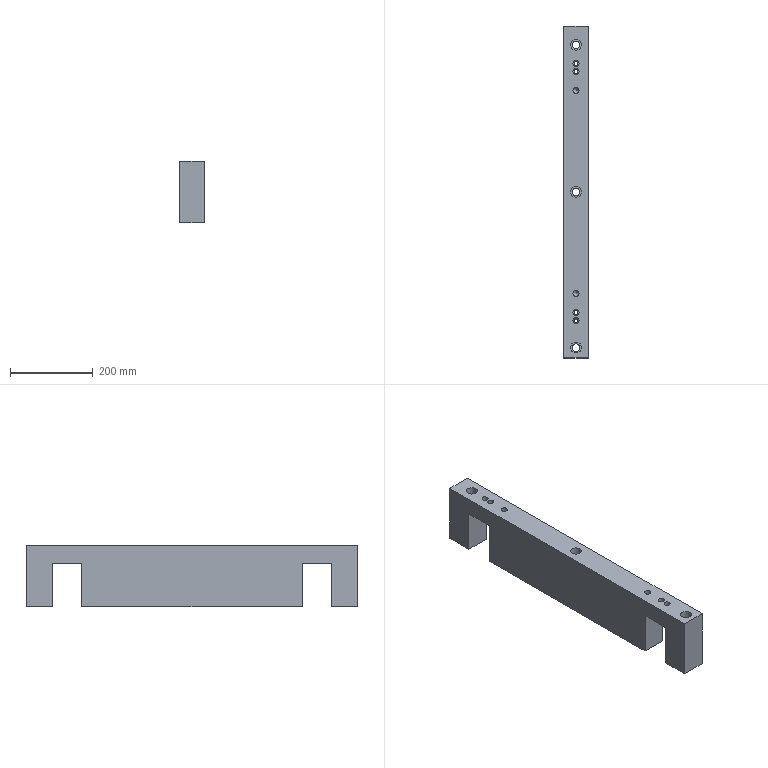Part | STEP file | lll_id2314_x_t | 1 solid | 39 faces | box 60 x 800 x 147.5 mm | volume 5972618 mm3 | plane 21 | cylinder 16 | cone 2 | commonest cylinder face diameters 9.009 x4 14.508 x4 18.009 x3 26.008 x3 14.506 x2
STEP:
#1=CARTESIAN_POINT('',(2157.253,-244.498,370.));
#2=VERTEX_POINT('',#1);
#3=CARTESIAN_POINT('',(2150.,-244.498,370.));
#4=DIRECTION('',(0.,0.,-1.));
#5=DIRECTION('',(1.,0.,0.));
#6=AXIS2_PLACEMENT_3D('',#3,#4,#5);
#7=CIRCLE('',#6,7.253);
#8=EDGE_CURVE('',#2,#2,#7,.T.);
#9=ORIENTED_EDGE('',*,*,#8,.T.);
#10=EDGE_LOOP('',(#9));
#11=FACE_BOUND('',#10,.T.);
#12=CARTESIAN_POINT('',(2157.253,244.498,370.));
#13=VERTEX_POINT('',#12);
#14=CARTESIAN_POINT('',(2150.,244.498,370.));
#15=DIRECTION('',(0.,0.,1.));
#16=DIRECTION('',(1.,0.,0.));
#17=AXIS2_PLACEMENT_3D('',#14,#15,#16);
#18=CIRCLE('',#17,7.253);
#19=EDGE_CURVE('',#13,#13,#18,.T.);
#20=ORIENTED_EDGE('',*,*,#19,.F.);
#21=EDGE_LOOP('',(#20));
#22=FACE_BOUND('',#21,.T.);
#23=CARTESIAN_POINT('',(2163.004,355.,370.));
#24=VERTEX_POINT('',#23);
#25=CARTESIAN_POINT('',(2150.,355.,370.));
#26=DIRECTION('',(0.,0.,-1.));
#27=DIRECTION('',(1.,0.,0.));
#28=AXIS2_PLACEMENT_3D('',#25,#26,#27);
#29=CIRCLE('',#28,13.004);
#30=EDGE_CURVE('',#24,#24,#29,.T.);
#31=ORIENTED_EDGE('',*,*,#30,.T.);
#32=EDGE_LOOP('',(#31));
#33=FACE_BOUND('',#32,.T.);
#34=CARTESIAN_POINT('',(2180.,400.,370.));
#35=VERTEX_POINT('',#34);
#36=CARTESIAN_POINT('',(2120.,400.,370.));
#37=VERTEX_POINT('',#36);
#38=CARTESIAN_POINT('',(6090.,400.,370.));
#39=DIRECTION('',(-1.,0.,0.));
#40=VECTOR('',#39,1.);
#41=LINE('',#38,#40);
#42=EDGE_CURVE('',#35,#37,#41,.T.);
#43=ORIENTED_EDGE('',*,*,#42,.T.);
#44=CARTESIAN_POINT('',(2120.,-400.,370.));
#45=VERTEX_POINT('',#44);
#46=CARTESIAN_POINT('',(2120.,600.,370.));
#47=DIRECTION('',(0.,-1.,0.));
#48=VECTOR('',#47,1.);
#49=LINE('',#46,#48);
#50=EDGE_CURVE('',#37,#45,#49,.T.);
#51=ORIENTED_EDGE('',*,*,#50,.T.);
#52=CARTESIAN_POINT('',(2180.,-400.,370.));
#53=VERTEX_POINT('',#52);
#54=CARTESIAN_POINT('',(2120.,-400.,370.));
#55=DIRECTION('',(1.,0.,0.));
#56=VECTOR('',#55,1.);
#57=LINE('',#54,#56);
#58=EDGE_CURVE('',#45,#53,#57,.T.);
#59=ORIENTED_EDGE('',*,*,#58,.T.);
#60=CARTESIAN_POINT('',(2180.,1.,370.));
#61=DIRECTION('',(0.,1.,0.));
#62=VECTOR('',#61,1.);
#63=LINE('',#60,#62);
#64=EDGE_CURVE('',#53,#35,#63,.T.);
#65=ORIENTED_EDGE('',*,*,#64,.T.);
#66=EDGE_LOOP('',(#43,#51,#59,#65));
#67=FACE_BOUND('',#66,.T.);
#68=CARTESIAN_POINT('',(2157.254,310.,370.));
#69=VERTEX_POINT('',#68);
#70=CARTESIAN_POINT('',(2150.,310.,370.));
#71=DIRECTION('',(0.,0.,-1.));
#72=DIRECTION('',(1.,0.,0.));
#73=AXIS2_PLACEMENT_3D('',#70,#71,#72);
#74=CIRCLE('',#73,7.254);
#75=EDGE_CURVE('',#69,#69,#74,.T.);
#76=ORIENTED_EDGE('',*,*,#75,.T.);
#77=EDGE_LOOP('',(#76));
#78=FACE_BOUND('',#77,.T.);
#79=CARTESIAN_POINT('',(2157.254,290.,370.));
#80=VERTEX_POINT('',#79);
#81=CARTESIAN_POINT('',(2150.,290.,370.));
#82=DIRECTION('',(0.,0.,-1.));
#83=DIRECTION('',(1.,0.,0.));
#84=AXIS2_PLACEMENT_3D('',#81,#82,#83);
#85=CIRCLE('',#84,7.254);
#86=EDGE_CURVE('',#80,#80,#85,.T.);
#87=ORIENTED_EDGE('',*,*,#86,.T.);
#88=EDGE_LOOP('',(#87));
#89=FACE_BOUND('',#88,.T.);
#90=CARTESIAN_POINT('',(2157.254,-290.498,370.));
#91=VERTEX_POINT('',#90);
#92=CARTESIAN_POINT('',(2150.,-290.498,370.));
#93=DIRECTION('',(0.,0.,-1.));
#94=DIRECTION('',(1.,0.,0.));
#95=AXIS2_PLACEMENT_3D('',#92,#93,#94);
#96=CIRCLE('',#95,7.254);
#97=EDGE_CURVE('',#91,#91,#96,.T.);
#98=ORIENTED_EDGE('',*,*,#97,.T.);
#99=EDGE_LOOP('',(#98));
#100=FACE_BOUND('',#99,.T.);
#101=CARTESIAN_POINT('',(2157.254,-310.498,370.));
#102=VERTEX_POINT('',#101);
#103=CARTESIAN_POINT('',(2150.,-310.498,370.));
#104=DIRECTION('',(0.,0.,-1.));
#105=DIRECTION('',(1.,0.,0.));
#106=AXIS2_PLACEMENT_3D('',#103,#104,#105);
#107=CIRCLE('',#106,7.254);
#108=EDGE_CURVE('',#102,#102,#107,.T.);
#109=ORIENTED_EDGE('',*,*,#108,.T.);
#110=EDGE_LOOP('',(#109));
#111=FACE_BOUND('',#110,.T.);
#112=CARTESIAN_POINT('',(2163.004,0.,370.));
#113=VERTEX_POINT('',#112);
#114=CARTESIAN_POINT('',(2150.,0.,370.));
#115=DIRECTION('',(0.,0.,-1.));
#116=DIRECTION('',(1.,0.,0.));
#117=AXIS2_PLACEMENT_3D('',#114,#115,#116);
#118=CIRCLE('',#117,13.004);
#119=EDGE_CURVE('',#113,#113,#118,.T.);
#120=ORIENTED_EDGE('',*,*,#119,.T.);
#121=EDGE_LOOP('',(#120));
#122=FACE_BOUND('',#121,.T.);
#123=CARTESIAN_POINT('',(2163.004,-375.,370.));
#124=VERTEX_POINT('',#123);
#125=CARTESIAN_POINT('',(2150.,-375.,370.));
#126=DIRECTION('',(0.,0.,1.));
#127=DIRECTION('',(1.,0.,0.));
#128=AXIS2_PLACEMENT_3D('',#125,#126,#127);
#129=CIRCLE('',#128,13.004);
#130=EDGE_CURVE('',#124,#124,#129,.T.);
#131=ORIENTED_EDGE('',*,*,#130,.F.);
#132=EDGE_LOOP('',(#131));
#133=FACE_BOUND('',#132,.T.);
#134=CARTESIAN_POINT('',(-66.315,1.,370.));
#135=DIRECTION('',(0.,0.,-1.));
#136=DIRECTION('',(1.,0.,0.));
#137=AXIS2_PLACEMENT_3D('',#134,#135,#136);
#138=PLANE('',#137);
#139=ADVANCED_FACE('',(#11,#22,#33,#67,#78,#89,#100,#111,#122,#133),#138,.F.);
#140=CARTESIAN_POINT('',(2140.995,0.,222.5));
#141=VERTEX_POINT('',#140);
#142=CARTESIAN_POINT('',(2150.,0.,222.5));
#143=DIRECTION('',(0.,0.,-1.));
#144=DIRECTION('',(-1.,0.,0.));
#145=AXIS2_PLACEMENT_3D('',#142,#143,#144);
#146=CIRCLE('',#145,9.005);
#147=EDGE_CURVE('',#141,#141,#146,.T.);
#148=ORIENTED_EDGE('',*,*,#147,.F.);
#149=EDGE_LOOP('',(#148));
#150=FACE_BOUND('',#149,.T.);
#151=CARTESIAN_POINT('',(2180.,265.249,222.5));
#152=VERTEX_POINT('',#151);
#153=CARTESIAN_POINT('',(2120.,265.249,222.5));
#154=VERTEX_POINT('',#153);
#155=CARTESIAN_POINT('',(-66.315,265.249,222.5));
#156=DIRECTION('',(-1.,0.,0.));
#157=VECTOR('',#156,1.);
#158=LINE('',#155,#157);
#159=EDGE_CURVE('',#152,#154,#158,.T.);
#160=ORIENTED_EDGE('',*,*,#159,.F.);
#161=CARTESIAN_POINT('',(2180.,-265.249,222.5));
#162=VERTEX_POINT('',#161);
#163=CARTESIAN_POINT('',(2180.,1.,222.5));
#164=DIRECTION('',(0.,-1.,0.));
#165=VECTOR('',#164,1.);
#166=LINE('',#163,#165);
#167=EDGE_CURVE('',#152,#162,#166,.T.);
#168=ORIENTED_EDGE('',*,*,#167,.T.);
#169=CARTESIAN_POINT('',(2120.,-265.249,222.5));
#170=VERTEX_POINT('',#169);
#171=CARTESIAN_POINT('',(-66.315,-265.249,222.5));
#172=DIRECTION('',(1.,0.,0.));
#173=VECTOR('',#172,1.);
#174=LINE('',#171,#173);
#175=EDGE_CURVE('',#170,#162,#174,.T.);
#176=ORIENTED_EDGE('',*,*,#175,.F.);
#177=CARTESIAN_POINT('',(2120.,600.,222.5));
#178=DIRECTION('',(0.,-1.,0.));
#179=VECTOR('',#178,1.);
#180=LINE('',#177,#179);
#181=EDGE_CURVE('',#154,#170,#180,.T.);
#182=ORIENTED_EDGE('',*,*,#181,.F.);
#183=EDGE_LOOP('',(#160,#168,#176,#182));
#184=FACE_BOUND('',#183,.T.);
#185=CARTESIAN_POINT('',(-66.315,1.,222.5));
#186=DIRECTION('',(0.,0.,-1.));
#187=DIRECTION('',(1.,0.,0.));
#188=AXIS2_PLACEMENT_3D('',#185,#186,#187);
#189=PLANE('',#188);
#190=ADVANCED_FACE('',(#150,#184),#189,.T.);
#191=CARTESIAN_POINT('',(2140.995,355.,222.5));
#192=VERTEX_POINT('',#191);
#193=CARTESIAN_POINT('',(2150.,355.,222.5));
#194=DIRECTION('',(0.,0.,-1.));
#195=DIRECTION('',(-1.,0.,0.));
#196=AXIS2_PLACEMENT_3D('',#193,#194,#195);
#197=CIRCLE('',#196,9.005);
#198=EDGE_CURVE('',#192,#192,#197,.T.);
#199=ORIENTED_EDGE('',*,*,#198,.F.);
#200=EDGE_LOOP('',(#199));
#201=FACE_BOUND('',#200,.T.);
#202=CARTESIAN_POINT('',(2120.,335.249,222.5));
#203=VERTEX_POINT('',#202);
#204=CARTESIAN_POINT('',(2180.,335.249,222.5));
#205=VERTEX_POINT('',#204);
#206=CARTESIAN_POINT('',(-66.315,335.249,222.5));
#207=DIRECTION('',(1.,0.,0.));
#208=VECTOR('',#207,1.);
#209=LINE('',#206,#208);
#210=EDGE_CURVE('',#203,#205,#209,.T.);
#211=ORIENTED_EDGE('',*,*,#210,.F.);
#212=CARTESIAN_POINT('',(2120.,400.,222.5));
#213=VERTEX_POINT('',#212);
#214=CARTESIAN_POINT('',(2120.,600.,222.5));
#215=DIRECTION('',(0.,-1.,0.));
#216=VECTOR('',#215,1.);
#217=LINE('',#214,#216);
#218=EDGE_CURVE('',#213,#203,#217,.T.);
#219=ORIENTED_EDGE('',*,*,#218,.F.);
#220=CARTESIAN_POINT('',(2180.,400.,222.5));
#221=VERTEX_POINT('',#220);
#222=CARTESIAN_POINT('',(6090.,400.,222.5));
#223=DIRECTION('',(-1.,0.,0.));
#224=VECTOR('',#223,1.);
#225=LINE('',#222,#224);
#226=EDGE_CURVE('',#221,#213,#225,.T.);
#227=ORIENTED_EDGE('',*,*,#226,.F.);
#228=CARTESIAN_POINT('',(2180.,1.,222.5));
#229=DIRECTION('',(0.,-1.,0.));
#230=VECTOR('',#229,1.);
#231=LINE('',#228,#230);
#232=EDGE_CURVE('',#221,#205,#231,.T.);
#233=ORIENTED_EDGE('',*,*,#232,.T.);
#234=EDGE_LOOP('',(#211,#219,#227,#233));
#235=FACE_BOUND('',#234,.T.);
#236=CARTESIAN_POINT('',(-66.315,1.,222.5));
#237=DIRECTION('',(0.,0.,-1.));
#238=DIRECTION('',(1.,0.,0.));
#239=AXIS2_PLACEMENT_3D('',#236,#237,#238);
#240=PLANE('',#239);
#241=ADVANCED_FACE('',(#201,#235),#240,.T.);
#242=CARTESIAN_POINT('',(2140.995,-375.,222.5));
#243=VERTEX_POINT('',#242);
#244=CARTESIAN_POINT('',(2150.,-375.,222.5));
#245=DIRECTION('',(0.,0.,-1.));
#246=DIRECTION('',(-1.,0.,0.));
#247=AXIS2_PLACEMENT_3D('',#244,#245,#246);
#248=CIRCLE('',#247,9.005);
#249=EDGE_CURVE('',#243,#243,#248,.T.);
#250=ORIENTED_EDGE('',*,*,#249,.F.);
#251=EDGE_LOOP('',(#250));
#252=FACE_BOUND('',#251,.T.);
#253=CARTESIAN_POINT('',(2180.,-335.249,222.5));
#254=VERTEX_POINT('',#253);
#255=CARTESIAN_POINT('',(2120.,-335.249,222.5));
#256=VERTEX_POINT('',#255);
#257=CARTESIAN_POINT('',(-66.315,-335.249,222.5));
#258=DIRECTION('',(-1.,0.,0.));
#259=VECTOR('',#258,1.);
#260=LINE('',#257,#259);
#261=EDGE_CURVE('',#254,#256,#260,.T.);
#262=ORIENTED_EDGE('',*,*,#261,.F.);
#263=CARTESIAN_POINT('',(2180.,-400.,222.5));
#264=VERTEX_POINT('',#263);
#265=CARTESIAN_POINT('',(2180.,1.,222.5));
#266=DIRECTION('',(0.,-1.,0.));
#267=VECTOR('',#266,1.);
#268=LINE('',#265,#267);
#269=EDGE_CURVE('',#254,#264,#268,.T.);
#270=ORIENTED_EDGE('',*,*,#269,.T.);
#271=CARTESIAN_POINT('',(2120.,-400.,222.5));
#272=VERTEX_POINT('',#271);
#273=CARTESIAN_POINT('',(2120.,-400.,222.5));
#274=DIRECTION('',(1.,0.,0.));
#275=VECTOR('',#274,1.);
#276=LINE('',#273,#275);
#277=EDGE_CURVE('',#272,#264,#276,.T.);
#278=ORIENTED_EDGE('',*,*,#277,.F.);
#279=CARTESIAN_POINT('',(2120.,600.,222.5));
#280=DIRECTION('',(0.,-1.,0.));
#281=VECTOR('',#280,1.);
#282=LINE('',#279,#281);
#283=EDGE_CURVE('',#256,#272,#282,.T.);
#284=ORIENTED_EDGE('',*,*,#283,.F.);
#285=EDGE_LOOP('',(#262,#270,#278,#284));
#286=FACE_BOUND('',#285,.T.);
#287=CARTESIAN_POINT('',(-66.315,1.,222.5));
#288=DIRECTION('',(0.,0.,-1.));
#289=DIRECTION('',(1.,0.,0.));
#290=AXIS2_PLACEMENT_3D('',#287,#288,#289);
#291=PLANE('',#290);
#292=ADVANCED_FACE('',(#252,#286),#291,.T.);
#293=CARTESIAN_POINT('',(2120.,-335.249,326.5));
#294=VERTEX_POINT('',#293);
#295=CARTESIAN_POINT('',(2120.,-265.249,326.5));
#296=VERTEX_POINT('',#295);
#297=CARTESIAN_POINT('',(2120.,-50.498,326.5));
#298=DIRECTION('',(0.,1.,0.));
#299=VECTOR('',#298,1.);
#300=LINE('',#297,#299);
#301=EDGE_CURVE('',#294,#296,#300,.T.);
#302=ORIENTED_EDGE('',*,*,#301,.F.);
#303=CARTESIAN_POINT('',(2120.,-335.249,363.5));
#304=DIRECTION('',(0.,0.,1.));
#305=VECTOR('',#304,1.);
#306=LINE('',#303,#305);
#307=EDGE_CURVE('',#256,#294,#306,.T.);
#308=ORIENTED_EDGE('',*,*,#307,.F.);
#309=ORIENTED_EDGE('',*,*,#283,.T.);
#310=CARTESIAN_POINT('',(2120.,-400.,310.));
#311=DIRECTION('',(0.,0.,-1.));
#312=VECTOR('',#311,1.);
#313=LINE('',#310,#312);
#314=EDGE_CURVE('',#45,#272,#313,.T.);
#315=ORIENTED_EDGE('',*,*,#314,.F.);
#316=ORIENTED_EDGE('',*,*,#50,.F.);
#317=CARTESIAN_POINT('',(2120.,400.,310.));
#318=DIRECTION('',(0.,0.,-1.));
#319=VECTOR('',#318,1.);
#320=LINE('',#317,#319);
#321=EDGE_CURVE('',#37,#213,#320,.T.);
#322=ORIENTED_EDGE('',*,*,#321,.T.);
#323=ORIENTED_EDGE('',*,*,#218,.T.);
#324=CARTESIAN_POINT('',(2120.,335.249,326.5));
#325=VERTEX_POINT('',#324);
#326=CARTESIAN_POINT('',(2120.,335.249,363.5));
#327=DIRECTION('',(0.,0.,-1.));
#328=VECTOR('',#327,1.);
#329=LINE('',#326,#328);
#330=EDGE_CURVE('',#325,#203,#329,.T.);
#331=ORIENTED_EDGE('',*,*,#330,.F.);
#332=CARTESIAN_POINT('',(2120.,265.249,326.5));
#333=VERTEX_POINT('',#332);
#334=CARTESIAN_POINT('',(2120.,550.,326.5));
#335=DIRECTION('',(0.,-1.,0.));
#336=VECTOR('',#335,1.);
#337=LINE('',#334,#336);
#338=EDGE_CURVE('',#325,#333,#337,.T.);
#339=ORIENTED_EDGE('',*,*,#338,.T.);
#340=CARTESIAN_POINT('',(2120.,265.249,363.5));
#341=DIRECTION('',(0.,0.,1.));
#342=VECTOR('',#341,1.);
#343=LINE('',#340,#342);
#344=EDGE_CURVE('',#154,#333,#343,.T.);
#345=ORIENTED_EDGE('',*,*,#344,.F.);
#346=ORIENTED_EDGE('',*,*,#181,.T.);
#347=CARTESIAN_POINT('',(2120.,-265.249,363.5));
#348=DIRECTION('',(0.,0.,-1.));
#349=VECTOR('',#348,1.);
#350=LINE('',#347,#349);
#351=EDGE_CURVE('',#296,#170,#350,.T.);
#352=ORIENTED_EDGE('',*,*,#351,.F.);
#353=EDGE_LOOP('',(#302,#308,#309,#315,#316,#322,#323,#331,#339,#345,#346,#352));
#354=FACE_OUTER_BOUND('',#353,.T.);
#355=CARTESIAN_POINT('',(2120.,600.,310.));
#356=DIRECTION('',(-1.,0.,0.));
#357=DIRECTION('',(0.,0.,-1.));
#358=AXIS2_PLACEMENT_3D('',#355,#356,#357);
#359=PLANE('',#358);
#360=ADVANCED_FACE('',(#354),#359,.T.);
#361=CARTESIAN_POINT('',(2180.,-400.,310.));
#362=DIRECTION('',(0.,0.,-1.));
#363=VECTOR('',#362,1.);
#364=LINE('',#361,#363);
#365=EDGE_CURVE('',#53,#264,#364,.T.);
#366=ORIENTED_EDGE('',*,*,#365,.F.);
#367=ORIENTED_EDGE('',*,*,#58,.F.);
#368=ORIENTED_EDGE('',*,*,#314,.T.);
#369=ORIENTED_EDGE('',*,*,#277,.T.);
#370=EDGE_LOOP('',(#366,#367,#368,#369));
#371=FACE_OUTER_BOUND('',#370,.T.);
#372=CARTESIAN_POINT('',(2120.,-400.,310.));
#373=DIRECTION('',(0.,-1.,0.));
#374=DIRECTION('',(0.,0.,-1.));
#375=AXIS2_PLACEMENT_3D('',#372,#373,#374);
#376=PLANE('',#375);
#377=ADVANCED_FACE('',(#371),#376,.T.);
#378=CARTESIAN_POINT('',(2180.,400.,310.));
#379=DIRECTION('',(0.,0.,1.));
#380=VECTOR('',#379,1.);
#381=LINE('',#378,#380);
#382=EDGE_CURVE('',#221,#35,#381,.T.);
#383=ORIENTED_EDGE('',*,*,#382,.F.);
#384=ORIENTED_EDGE('',*,*,#226,.T.);
#385=ORIENTED_EDGE('',*,*,#321,.F.);
#386=ORIENTED_EDGE('',*,*,#42,.F.);
#387=EDGE_LOOP('',(#383,#384,#385,#386));
#388=FACE_OUTER_BOUND('',#387,.T.);
#389=CARTESIAN_POINT('',(6090.,400.,310.));
#390=DIRECTION('',(0.,1.,0.));
#391=DIRECTION('',(0.,0.,1.));
#392=AXIS2_PLACEMENT_3D('',#389,#390,#391);
#393=PLANE('',#392);
#394=ADVANCED_FACE('',(#388),#393,.T.);
#395=CARTESIAN_POINT('',(2180.,-335.249,326.5));
#396=VERTEX_POINT('',#395);
#397=CARTESIAN_POINT('',(2180.,-335.249,294.75));
#398=DIRECTION('',(0.,0.,1.));
#399=VECTOR('',#398,1.);
#400=LINE('',#397,#399);
#401=EDGE_CURVE('',#254,#396,#400,.T.);
#402=ORIENTED_EDGE('',*,*,#401,.T.);
#403=CARTESIAN_POINT('',(2180.,-265.249,326.5));
#404=VERTEX_POINT('',#403);
#405=CARTESIAN_POINT('',(2180.,-650.498,326.5));
#406=DIRECTION('',(0.,-1.,0.));
#407=VECTOR('',#406,1.);
#408=LINE('',#405,#407);
#409=EDGE_CURVE('',#404,#396,#408,.T.);
#410=ORIENTED_EDGE('',*,*,#409,.F.);
#411=CARTESIAN_POINT('',(2180.,-265.249,294.75));
#412=DIRECTION('',(0.,0.,-1.));
#413=VECTOR('',#412,1.);
#414=LINE('',#411,#413);
#415=EDGE_CURVE('',#404,#162,#414,.T.);
#416=ORIENTED_EDGE('',*,*,#415,.T.);
#417=ORIENTED_EDGE('',*,*,#167,.F.);
#418=CARTESIAN_POINT('',(2180.,265.249,326.5));
#419=VERTEX_POINT('',#418);
#420=CARTESIAN_POINT('',(2180.,265.249,294.75));
#421=DIRECTION('',(0.,0.,1.));
#422=VECTOR('',#421,1.);
#423=LINE('',#420,#422);
#424=EDGE_CURVE('',#152,#419,#423,.T.);
#425=ORIENTED_EDGE('',*,*,#424,.T.);
#426=CARTESIAN_POINT('',(2180.,335.249,326.5));
#427=VERTEX_POINT('',#426);
#428=CARTESIAN_POINT('',(2180.,-50.,326.5));
#429=DIRECTION('',(0.,-1.,0.));
#430=VECTOR('',#429,1.);
#431=LINE('',#428,#430);
#432=EDGE_CURVE('',#427,#419,#431,.T.);
#433=ORIENTED_EDGE('',*,*,#432,.F.);
#434=CARTESIAN_POINT('',(2180.,335.249,294.75));
#435=DIRECTION('',(0.,0.,-1.));
#436=VECTOR('',#435,1.);
#437=LINE('',#434,#436);
#438=EDGE_CURVE('',#427,#205,#437,.T.);
#439=ORIENTED_EDGE('',*,*,#438,.T.);
#440=ORIENTED_EDGE('',*,*,#232,.F.);
#441=ORIENTED_EDGE('',*,*,#382,.T.);
#442=ORIENTED_EDGE('',*,*,#64,.F.);
#443=ORIENTED_EDGE('',*,*,#365,.T.);
#444=ORIENTED_EDGE('',*,*,#269,.F.);
#445=EDGE_LOOP('',(#402,#410,#416,#417,#425,#433,#439,#440,#441,#442,#443,#444));
#446=FACE_OUTER_BOUND('',#445,.T.);
#447=CARTESIAN_POINT('',(2180.,0.,241.25));
#448=DIRECTION('',(-1.,0.,0.));
#449=DIRECTION('',(0.,0.,-1.));
#450=AXIS2_PLACEMENT_3D('',#447,#448,#449);
#451=PLANE('',#450);
#452=ADVANCED_FACE('',(#446),#451,.F.);
#453=ORIENTED_EDGE('',*,*,#351,.T.);
#454=ORIENTED_EDGE('',*,*,#175,.T.);
#455=ORIENTED_EDGE('',*,*,#415,.F.);
#456=CARTESIAN_POINT('',(2150.,-265.249,326.5));
#457=DIRECTION('',(-1.,0.,0.));
#458=VECTOR('',#457,1.);
#459=LINE('',#456,#458);
#460=EDGE_CURVE('',#404,#296,#459,.T.);
#461=ORIENTED_EDGE('',*,*,#460,.T.);
#462=EDGE_LOOP('',(#453,#454,#455,#461));
#463=FACE_OUTER_BOUND('',#462,.T.);
#464=CARTESIAN_POINT('',(2150.,-265.249,130.));
#465=DIRECTION('',(0.,1.,0.));
#466=DIRECTION('',(0.,0.,-1.));
#467=AXIS2_PLACEMENT_3D('',#464,#465,#466);
#468=PLANE('',#467);
#469=ADVANCED_FACE('',(#463),#468,.F.);
#470=ORIENTED_EDGE('',*,*,#307,.T.);
#471=CARTESIAN_POINT('',(2150.,-335.249,326.5));
#472=DIRECTION('',(1.,0.,0.));
#473=VECTOR('',#472,1.);
#474=LINE('',#471,#473);
#475=EDGE_CURVE('',#294,#396,#474,.T.);
#476=ORIENTED_EDGE('',*,*,#475,.T.);
#477=ORIENTED_EDGE('',*,*,#401,.F.);
#478=ORIENTED_EDGE('',*,*,#261,.T.);
#479=EDGE_LOOP('',(#470,#476,#477,#478));
#480=FACE_OUTER_BOUND('',#479,.T.);
#481=CARTESIAN_POINT('',(2150.,-335.249,130.));
#482=DIRECTION('',(0.,-1.,0.));
#483=DIRECTION('',(0.,0.,1.));
#484=AXIS2_PLACEMENT_3D('',#481,#482,#483);
#485=PLANE('',#484);
#486=ADVANCED_FACE('',(#480),#485,.F.);
#487=ORIENTED_EDGE('',*,*,#344,.T.);
#488=CARTESIAN_POINT('',(2150.,265.249,326.5));
#489=DIRECTION('',(1.,0.,0.));
#490=VECTOR('',#489,1.);
#491=LINE('',#488,#490);
#492=EDGE_CURVE('',#333,#419,#491,.T.);
#493=ORIENTED_EDGE('',*,*,#492,.T.);
#494=ORIENTED_EDGE('',*,*,#424,.F.);
#495=ORIENTED_EDGE('',*,*,#159,.T.);
#496=EDGE_LOOP('',(#487,#493,#494,#495));
#497=FACE_OUTER_BOUND('',#496,.T.);
#498=CARTESIAN_POINT('',(2150.,265.249,130.));
#499=DIRECTION('',(0.,-1.,0.));
#500=DIRECTION('',(0.,0.,-1.));
#501=AXIS2_PLACEMENT_3D('',#498,#499,#500);
#502=PLANE('',#501);
#503=ADVANCED_FACE('',(#497),#502,.F.);
#504=ORIENTED_EDGE('',*,*,#330,.T.);
#505=ORIENTED_EDGE('',*,*,#210,.T.);
#506=ORIENTED_EDGE('',*,*,#438,.F.);
#507=CARTESIAN_POINT('',(2150.,335.249,326.5));
#508=DIRECTION('',(-1.,0.,0.));
#509=VECTOR('',#508,1.);
#510=LINE('',#507,#509);
#511=EDGE_CURVE('',#427,#325,#510,.T.);
#512=ORIENTED_EDGE('',*,*,#511,.T.);
#513=EDGE_LOOP('',(#504,#505,#506,#512));
#514=FACE_OUTER_BOUND('',#513,.T.);
#515=CARTESIAN_POINT('',(2150.,335.249,130.));
#516=DIRECTION('',(0.,1.,0.));
#517=DIRECTION('',(0.,0.,1.));
#518=AXIS2_PLACEMENT_3D('',#515,#516,#517);
#519=PLANE('',#518);
#520=ADVANCED_FACE('',(#514),#519,.F.);
#521=CARTESIAN_POINT('',(2157.254,290.,351.5));
#522=VERTEX_POINT('',#521);
#523=CARTESIAN_POINT('',(2150.,290.,351.5));
#524=DIRECTION('',(0.,0.,-1.));
#525=DIRECTION('',(1.,0.,0.));
#526=AXIS2_PLACEMENT_3D('',#523,#524,#525);
#527=CIRCLE('',#526,7.254);
#528=EDGE_CURVE('',#522,#522,#527,.T.);
#529=ORIENTED_EDGE('',*,*,#528,.T.);
#530=EDGE_LOOP('',(#529));
#531=FACE_BOUND('',#530,.T.);
#532=ORIENTED_EDGE('',*,*,#86,.F.);
#533=EDGE_LOOP('',(#532));
#534=FACE_BOUND('',#533,.T.);
#535=CARTESIAN_POINT('',(2150.,290.,370.));
#536=DIRECTION('',(0.,0.,-1.));
#537=DIRECTION('',(1.,0.,0.));
#538=AXIS2_PLACEMENT_3D('',#535,#536,#537);
#539=CYLINDRICAL_SURFACE('',#538,7.254);
#540=ADVANCED_FACE('',(#531,#534),#539,.F.);
#541=CARTESIAN_POINT('',(2157.254,310.,351.5));
#542=VERTEX_POINT('',#541);
#543=CARTESIAN_POINT('',(2150.,310.,351.5));
#544=DIRECTION('',(0.,0.,-1.));
#545=DIRECTION('',(1.,0.,0.));
#546=AXIS2_PLACEMENT_3D('',#543,#544,#545);
#547=CIRCLE('',#546,7.254);
#548=EDGE_CURVE('',#542,#542,#547,.T.);
#549=ORIENTED_EDGE('',*,*,#548,.T.);
#550=EDGE_LOOP('',(#549));
#551=FACE_BOUND('',#550,.T.);
#552=ORIENTED_EDGE('',*,*,#75,.F.);
#553=EDGE_LOOP('',(#552));
#554=FACE_BOUND('',#553,.T.);
#555=CARTESIAN_POINT('',(2150.,310.,370.));
#556=DIRECTION('',(0.,0.,-1.));
#557=DIRECTION('',(1.,0.,0.));
#558=AXIS2_PLACEMENT_3D('',#555,#556,#557);
#559=CYLINDRICAL_SURFACE('',#558,7.254);
#560=ADVANCED_FACE('',(#551,#554),#559,.F.);
#561=CARTESIAN_POINT('',(2145.495,310.,351.5));
#562=VERTEX_POINT('',#561);
#563=CARTESIAN_POINT('',(2150.,310.,351.5));
#564=DIRECTION('',(0.,0.,-1.));
#565=DIRECTION('',(-1.,0.,0.));
#566=AXIS2_PLACEMENT_3D('',#563,#564,#565);
#567=CIRCLE('',#566,4.505);
#568=EDGE_CURVE('',#562,#562,#567,.T.);
#569=ORIENTED_EDGE('',*,*,#568,.T.);
#570=EDGE_LOOP('',(#569));
#571=FACE_BOUND('',#570,.T.);
#572=ORIENTED_EDGE('',*,*,#548,.F.);
#573=EDGE_LOOP('',(#572));
#574=FACE_BOUND('',#573,.T.);
#575=CARTESIAN_POINT('',(2150.,310.,351.5));
#576=DIRECTION('',(0.,0.,-1.));
#577=DIRECTION('',(-1.,0.,0.));
#578=AXIS2_PLACEMENT_3D('',#575,#576,#577);
#579=PLANE('',#578);
#580=ADVANCED_FACE('',(#571,#574),#579,.F.);
#581=CARTESIAN_POINT('',(2145.495,290.,351.5));
#582=VERTEX_POINT('',#581);
#583=CARTESIAN_POINT('',(2150.,290.,351.5));
#584=DIRECTION('',(0.,0.,-1.));
#585=DIRECTION('',(-1.,0.,0.));
#586=AXIS2_PLACEMENT_3D('',#583,#584,#585);
#587=CIRCLE('',#586,4.505);
#588=EDGE_CURVE('',#582,#582,#587,.T.);
#589=ORIENTED_EDGE('',*,*,#588,.F.);
#590=EDGE_LOOP('',(#589));
#591=FACE_BOUND('',#590,.T.);
#592=CARTESIAN_POINT('',(2154.505,290.,326.5));
#593=VERTEX_POINT('',#592);
#594=CARTESIAN_POINT('',(2150.,290.,326.5));
#595=DIRECTION('',(0.,0.,1.));
#596=DIRECTION('',(1.,0.,0.));
#597=AXIS2_PLACEMENT_3D('',#594,#595,#596);
#598=CIRCLE('',#597,4.505);
#599=EDGE_CURVE('',#593,#593,#598,.T.);
#600=ORIENTED_EDGE('',*,*,#599,.F.);
#601=EDGE_LOOP('',(#600));
#602=FACE_BOUND('',#601,.T.);
#603=CARTESIAN_POINT('',(2150.,290.,370.));
#604=DIRECTION('',(0.,0.,-1.));
#605=DIRECTION('',(1.,0.,0.));
#606=AXIS2_PLACEMENT_3D('',#603,#604,#605);
#607=CYLINDRICAL_SURFACE('',#606,4.505);
#608=ADVANCED_FACE('',(#591,#602),#607,.F.);
#609=ORIENTED_EDGE('',*,*,#588,.T.);
#610=EDGE_LOOP('',(#609));
#611=FACE_BOUND('',#610,.T.);
#612=ORIENTED_EDGE('',*,*,#528,.F.);
#613=EDGE_LOOP('',(#612));
#614=FACE_BOUND('',#613,.T.);
#615=CARTESIAN_POINT('',(2150.,290.,351.5));
#616=DIRECTION('',(0.,0.,-1.));
#617=DIRECTION('',(-1.,0.,0.));
#618=AXIS2_PLACEMENT_3D('',#615,#616,#617);
#619=PLANE('',#618);
#620=ADVANCED_FACE('',(#611,#614),#619,.F.);
#621=ORIENTED_EDGE('',*,*,#599,.T.);
#622=EDGE_LOOP('',(#621));
#623=FACE_BOUND('',#622,.T.);
#624=CARTESIAN_POINT('',(2154.505,310.,326.5));
#625=VERTEX_POINT('',#624);
#626=CARTESIAN_POINT('',(2150.,310.,326.5));
#627=DIRECTION('',(0.,0.,1.));
#628=DIRECTION('',(1.,0.,0.));
#629=AXIS2_PLACEMENT_3D('',#626,#627,#628);
#630=CIRCLE('',#629,4.505);
#631=EDGE_CURVE('',#625,#625,#630,.T.);
#632=ORIENTED_EDGE('',*,*,#631,.T.);
#633=EDGE_LOOP('',(#632));
#634=FACE_BOUND('',#633,.T.);
#635=ORIENTED_EDGE('',*,*,#338,.F.);
#636=ORIENTED_EDGE('',*,*,#511,.F.);
#637=ORIENTED_EDGE('',*,*,#432,.T.);
#638=ORIENTED_EDGE('',*,*,#492,.F.);
#639=EDGE_LOOP('',(#635,#636,#637,#638));
#640=FACE_BOUND('',#639,.T.);
#641=CARTESIAN_POINT('',(2150.,300.249,326.5));
#642=DIRECTION('',(0.,0.,1.));
#643=DIRECTION('',(1.,0.,0.));
#644=AXIS2_PLACEMENT_3D('',#641,#642,#643);
#645=PLANE('',#644);
#646=ADVANCED_FACE('',(#623,#634,#640),#645,.F.);
#647=ORIENTED_EDGE('',*,*,#568,.F.);
#648=EDGE_LOOP('',(#647));
#649=FACE_BOUND('',#648,.T.);
#650=ORIENTED_EDGE('',*,*,#631,.F.);
#651=EDGE_LOOP('',(#650));
#652=FACE_BOUND('',#651,.T.);
#653=CARTESIAN_POINT('',(2150.,310.,370.));
#654=DIRECTION('',(0.,0.,-1.));
#655=DIRECTION('',(1.,0.,0.));
#656=AXIS2_PLACEMENT_3D('',#653,#654,#655);
#657=CYLINDRICAL_SURFACE('',#656,4.505);
#658=ADVANCED_FACE('',(#649,#652),#657,.F.);
#659=CARTESIAN_POINT('',(2157.254,-310.498,351.5));
#660=VERTEX_POINT('',#659);
#661=CARTESIAN_POINT('',(2150.,-310.498,351.5));
#662=DIRECTION('',(0.,0.,-1.));
#663=DIRECTION('',(1.,0.,0.));
#664=AXIS2_PLACEMENT_3D('',#661,#662,#663);
#665=CIRCLE('',#664,7.254);
#666=EDGE_CURVE('',#660,#660,#665,.T.);
#667=ORIENTED_EDGE('',*,*,#666,.T.);
#668=EDGE_LOOP('',(#667));
#669=FACE_BOUND('',#668,.T.);
#670=ORIENTED_EDGE('',*,*,#108,.F.);
#671=EDGE_LOOP('',(#670));
#672=FACE_BOUND('',#671,.T.);
#673=CARTESIAN_POINT('',(2150.,-310.498,370.));
#674=DIRECTION('',(0.,0.,-1.));
#675=DIRECTION('',(1.,0.,0.));
#676=AXIS2_PLACEMENT_3D('',#673,#674,#675);
#677=CYLINDRICAL_SURFACE('',#676,7.254);
#678=ADVANCED_FACE('',(#669,#672),#677,.F.);
#679=CARTESIAN_POINT('',(2157.254,-290.498,351.5));
#680=VERTEX_POINT('',#679);
#681=CARTESIAN_POINT('',(2150.,-290.498,351.5));
#682=DIRECTION('',(0.,0.,-1.));
#683=DIRECTION('',(1.,0.,0.));
#684=AXIS2_PLACEMENT_3D('',#681,#682,#683);
#685=CIRCLE('',#684,7.254);
#686=EDGE_CURVE('',#680,#680,#685,.T.);
#687=ORIENTED_EDGE('',*,*,#686,.T.);
#688=EDGE_LOOP('',(#687));
#689=FACE_BOUND('',#688,.T.);
#690=ORIENTED_EDGE('',*,*,#97,.F.);
#691=EDGE_LOOP('',(#690));
#692=FACE_BOUND('',#691,.T.);
#693=CARTESIAN_POINT('',(2150.,-290.498,370.));
#694=DIRECTION('',(0.,0.,-1.));
#695=DIRECTION('',(1.,0.,0.));
#696=AXIS2_PLACEMENT_3D('',#693,#694,#695);
#697=CYLINDRICAL_SURFACE('',#696,7.254);
#698=ADVANCED_FACE('',(#689,#692),#697,.F.);
#699=CARTESIAN_POINT('',(2145.495,-290.498,351.5));
#700=VERTEX_POINT('',#699);
#701=CARTESIAN_POINT('',(2150.,-290.498,351.5));
#702=DIRECTION('',(0.,0.,-1.));
#703=DIRECTION('',(-1.,0.,0.));
#704=AXIS2_PLACEMENT_3D('',#701,#702,#703);
#705=CIRCLE('',#704,4.505);
#706=EDGE_CURVE('',#700,#700,#705,.T.);
#707=ORIENTED_EDGE('',*,*,#706,.T.);
#708=EDGE_LOOP('',(#707));
#709=FACE_BOUND('',#708,.T.);
#710=ORIENTED_EDGE('',*,*,#686,.F.);
#711=EDGE_LOOP('',(#710));
#712=FACE_BOUND('',#711,.T.);
#713=CARTESIAN_POINT('',(2150.,-290.498,351.5));
#714=DIRECTION('',(0.,0.,-1.));
#715=DIRECTION('',(-1.,0.,0.));
#716=AXIS2_PLACEMENT_3D('',#713,#714,#715);
#717=PLANE('',#716);
#718=ADVANCED_FACE('',(#709,#712),#717,.F.);
#719=CARTESIAN_POINT('',(2145.495,-310.498,351.5));
#720=VERTEX_POINT('',#719);
#721=CARTESIAN_POINT('',(2150.,-310.498,351.5));
#722=DIRECTION('',(0.,0.,-1.));
#723=DIRECTION('',(-1.,0.,0.));
#724=AXIS2_PLACEMENT_3D('',#721,#722,#723);
#725=CIRCLE('',#724,4.505);
#726=EDGE_CURVE('',#720,#720,#725,.T.);
#727=ORIENTED_EDGE('',*,*,#726,.F.);
#728=EDGE_LOOP('',(#727));
#729=FACE_BOUND('',#728,.T.);
#730=CARTESIAN_POINT('',(2154.505,-310.498,326.5));
#731=VERTEX_POINT('',#730);
#732=CARTESIAN_POINT('',(2150.,-310.498,326.5));
#733=DIRECTION('',(0.,0.,1.));
#734=DIRECTION('',(1.,0.,0.));
#735=AXIS2_PLACEMENT_3D('',#732,#733,#734);
#736=CIRCLE('',#735,4.505);
#737=EDGE_CURVE('',#731,#731,#736,.T.);
#738=ORIENTED_EDGE('',*,*,#737,.F.);
#739=EDGE_LOOP('',(#738));
#740=FACE_BOUND('',#739,.T.);
#741=CARTESIAN_POINT('',(2150.,-310.498,370.));
#742=DIRECTION('',(0.,0.,-1.));
#743=DIRECTION('',(1.,0.,0.));
#744=AXIS2_PLACEMENT_3D('',#741,#742,#743);
#745=CYLINDRICAL_SURFACE('',#744,4.505);
#746=ADVANCED_FACE('',(#729,#740),#745,.F.);
#747=ORIENTED_EDGE('',*,*,#726,.T.);
#748=EDGE_LOOP('',(#747));
#749=FACE_BOUND('',#748,.T.);
#750=ORIENTED_EDGE('',*,*,#666,.F.);
#751=EDGE_LOOP('',(#750));
#752=FACE_BOUND('',#751,.T.);
#753=CARTESIAN_POINT('',(2150.,-310.498,351.5));
#754=DIRECTION('',(0.,0.,-1.));
#755=DIRECTION('',(-1.,0.,0.));
#756=AXIS2_PLACEMENT_3D('',#753,#754,#755);
#757=PLANE('',#756);
#758=ADVANCED_FACE('',(#749,#752),#757,.F.);
#759=ORIENTED_EDGE('',*,*,#737,.T.);
#760=EDGE_LOOP('',(#759));
#761=FACE_BOUND('',#760,.T.);
#762=CARTESIAN_POINT('',(2154.505,-290.498,326.5));
#763=VERTEX_POINT('',#762);
#764=CARTESIAN_POINT('',(2150.,-290.498,326.5));
#765=DIRECTION('',(0.,0.,1.));
#766=DIRECTION('',(1.,0.,0.));
#767=AXIS2_PLACEMENT_3D('',#764,#765,#766);
#768=CIRCLE('',#767,4.505);
#769=EDGE_CURVE('',#763,#763,#768,.T.);
#770=ORIENTED_EDGE('',*,*,#769,.T.);
#771=EDGE_LOOP('',(#770));
#772=FACE_BOUND('',#771,.T.);
#773=ORIENTED_EDGE('',*,*,#301,.T.);
#774=ORIENTED_EDGE('',*,*,#460,.F.);
#775=ORIENTED_EDGE('',*,*,#409,.T.);
#776=ORIENTED_EDGE('',*,*,#475,.F.);
#777=EDGE_LOOP('',(#773,#774,#775,#776));
#778=FACE_BOUND('',#777,.T.);
#779=CARTESIAN_POINT('',(2150.,-300.249,326.5));
#780=DIRECTION('',(0.,0.,1.));
#781=DIRECTION('',(1.,0.,0.));
#782=AXIS2_PLACEMENT_3D('',#779,#780,#781);
#783=PLANE('',#782);
#784=ADVANCED_FACE('',(#761,#772,#778),#783,.F.);
#785=ORIENTED_EDGE('',*,*,#706,.F.);
#786=EDGE_LOOP('',(#785));
#787=FACE_BOUND('',#786,.T.);
#788=ORIENTED_EDGE('',*,*,#769,.F.);
#789=EDGE_LOOP('',(#788));
#790=FACE_BOUND('',#789,.T.);
#791=CARTESIAN_POINT('',(2150.,-290.498,370.));
#792=DIRECTION('',(0.,0.,-1.));
#793=DIRECTION('',(1.,0.,0.));
#794=AXIS2_PLACEMENT_3D('',#791,#792,#793);
#795=CYLINDRICAL_SURFACE('',#794,4.505);
#796=ADVANCED_FACE('',(#787,#790),#795,.F.);
#797=ORIENTED_EDGE('',*,*,#147,.T.);
#798=EDGE_LOOP('',(#797));
#799=FACE_BOUND('',#798,.T.);
#800=CARTESIAN_POINT('',(2140.995,0.,262.5));
#801=VERTEX_POINT('',#800);
#802=CARTESIAN_POINT('',(2150.,0.,262.5));
#803=DIRECTION('',(0.,0.,-1.));
#804=DIRECTION('',(-1.,0.,0.));
#805=AXIS2_PLACEMENT_3D('',#802,#803,#804);
#806=CIRCLE('',#805,9.005);
#807=EDGE_CURVE('',#801,#801,#806,.T.);
#808=ORIENTED_EDGE('',*,*,#807,.F.);
#809=EDGE_LOOP('',(#808));
#810=FACE_BOUND('',#809,.T.);
#811=CARTESIAN_POINT('',(2150.,0.,422.));
#812=DIRECTION('',(0.,0.,-1.));
#813=DIRECTION('',(1.,0.,0.));
#814=AXIS2_PLACEMENT_3D('',#811,#812,#813);
#815=CYLINDRICAL_SURFACE('',#814,9.005);
#816=ADVANCED_FACE('',(#799,#810),#815,.F.);
#817=ORIENTED_EDGE('',*,*,#807,.T.);
#818=EDGE_LOOP('',(#817));
#819=FACE_BOUND('',#818,.T.);
#820=CARTESIAN_POINT('',(2163.004,0.,262.5));
#821=VERTEX_POINT('',#820);
#822=CARTESIAN_POINT('',(2150.,0.,262.5));
#823=DIRECTION('',(0.,0.,-1.));
#824=DIRECTION('',(1.,0.,0.));
#825=AXIS2_PLACEMENT_3D('',#822,#823,#824);
#826=CIRCLE('',#825,13.004);
#827=EDGE_CURVE('',#821,#821,#826,.T.);
#828=ORIENTED_EDGE('',*,*,#827,.F.);
#829=EDGE_LOOP('',(#828));
#830=FACE_BOUND('',#829,.T.);
#831=CARTESIAN_POINT('',(2150.,0.,262.5));
#832=DIRECTION('',(0.,0.,-1.));
#833=DIRECTION('',(-1.,0.,0.));
#834=AXIS2_PLACEMENT_3D('',#831,#832,#833);
#835=PLANE('',#834);
#836=ADVANCED_FACE('',(#819,#830),#835,.F.);
#837=ORIENTED_EDGE('',*,*,#827,.T.);
#838=EDGE_LOOP('',(#837));
#839=FACE_BOUND('',#838,.T.);
#840=ORIENTED_EDGE('',*,*,#119,.F.);
#841=EDGE_LOOP('',(#840));
#842=FACE_BOUND('',#841,.T.);
#843=CARTESIAN_POINT('',(2150.,0.,370.));
#844=DIRECTION('',(0.,0.,-1.));
#845=DIRECTION('',(1.,0.,0.));
#846=AXIS2_PLACEMENT_3D('',#843,#844,#845);
#847=CYLINDRICAL_SURFACE('',#846,13.004);
#848=ADVANCED_FACE('',(#839,#842),#847,.F.);
#849=ORIENTED_EDGE('',*,*,#249,.T.);
#850=EDGE_LOOP('',(#849));
#851=FACE_BOUND('',#850,.T.);
#852=CARTESIAN_POINT('',(2140.995,-375.,262.5));
#853=VERTEX_POINT('',#852);
#854=CARTESIAN_POINT('',(2150.,-375.,262.5));
#855=DIRECTION('',(0.,0.,1.));
#856=DIRECTION('',(-1.,0.,0.));
#857=AXIS2_PLACEMENT_3D('',#854,#855,#856);
#858=CIRCLE('',#857,9.005);
#859=EDGE_CURVE('',#853,#853,#858,.T.);
#860=ORIENTED_EDGE('',*,*,#859,.T.);
#861=EDGE_LOOP('',(#860));
#862=FACE_BOUND('',#861,.T.);
#863=CARTESIAN_POINT('',(2150.,-375.,422.));
#864=DIRECTION('',(0.,0.,-1.));
#865=DIRECTION('',(1.,0.,0.));
#866=AXIS2_PLACEMENT_3D('',#863,#864,#865);
#867=CYLINDRICAL_SURFACE('',#866,9.005);
#868=ADVANCED_FACE('',(#851,#862),#867,.F.);
#869=ORIENTED_EDGE('',*,*,#859,.F.);
#870=EDGE_LOOP('',(#869));
#871=FACE_BOUND('',#870,.T.);
#872=CARTESIAN_POINT('',(2163.004,-375.,262.5));
#873=VERTEX_POINT('',#872);
#874=CARTESIAN_POINT('',(2150.,-375.,262.5));
#875=DIRECTION('',(0.,0.,1.));
#876=DIRECTION('',(1.,0.,0.));
#877=AXIS2_PLACEMENT_3D('',#874,#875,#876);
#878=CIRCLE('',#877,13.004);
#879=EDGE_CURVE('',#873,#873,#878,.T.);
#880=ORIENTED_EDGE('',*,*,#879,.T.);
#881=EDGE_LOOP('',(#880));
#882=FACE_BOUND('',#881,.T.);
#883=CARTESIAN_POINT('',(2150.,-375.,262.5));
#884=DIRECTION('',(0.,0.,-1.));
#885=DIRECTION('',(-1.,0.,0.));
#886=AXIS2_PLACEMENT_3D('',#883,#884,#885);
#887=PLANE('',#886);
#888=ADVANCED_FACE('',(#871,#882),#887,.F.);
#889=ORIENTED_EDGE('',*,*,#879,.F.);
#890=EDGE_LOOP('',(#889));
#891=FACE_BOUND('',#890,.T.);
#892=ORIENTED_EDGE('',*,*,#130,.T.);
#893=EDGE_LOOP('',(#892));
#894=FACE_BOUND('',#893,.T.);
#895=CARTESIAN_POINT('',(2150.,-375.,370.));
#896=DIRECTION('',(0.,0.,-1.));
#897=DIRECTION('',(1.,0.,0.));
#898=AXIS2_PLACEMENT_3D('',#895,#896,#897);
#899=CYLINDRICAL_SURFACE('',#898,13.004);
#900=ADVANCED_FACE('',(#891,#894),#899,.F.);
#901=ORIENTED_EDGE('',*,*,#198,.T.);
#902=EDGE_LOOP('',(#901));
#903=FACE_BOUND('',#902,.T.);
#904=CARTESIAN_POINT('',(2140.995,355.,262.5));
#905=VERTEX_POINT('',#904);
#906=CARTESIAN_POINT('',(2150.,355.,262.5));
#907=DIRECTION('',(0.,0.,-1.));
#908=DIRECTION('',(-1.,0.,0.));
#909=AXIS2_PLACEMENT_3D('',#906,#907,#908);
#910=CIRCLE('',#909,9.005);
#911=EDGE_CURVE('',#905,#905,#910,.T.);
#912=ORIENTED_EDGE('',*,*,#911,.F.);
#913=EDGE_LOOP('',(#912));
#914=FACE_BOUND('',#913,.T.);
#915=CARTESIAN_POINT('',(2150.,355.,422.));
#916=DIRECTION('',(0.,0.,-1.));
#917=DIRECTION('',(1.,0.,0.));
#918=AXIS2_PLACEMENT_3D('',#915,#916,#917);
#919=CYLINDRICAL_SURFACE('',#918,9.005);
#920=ADVANCED_FACE('',(#903,#914),#919,.F.);
#921=ORIENTED_EDGE('',*,*,#911,.T.);
#922=EDGE_LOOP('',(#921));
#923=FACE_BOUND('',#922,.T.);
#924=CARTESIAN_POINT('',(2163.004,355.,262.5));
#925=VERTEX_POINT('',#924);
#926=CARTESIAN_POINT('',(2150.,355.,262.5));
#927=DIRECTION('',(0.,0.,-1.));
#928=DIRECTION('',(1.,0.,0.));
#929=AXIS2_PLACEMENT_3D('',#926,#927,#928);
#930=CIRCLE('',#929,13.004);
#931=EDGE_CURVE('',#925,#925,#930,.T.);
#932=ORIENTED_EDGE('',*,*,#931,.F.);
#933=EDGE_LOOP('',(#932));
#934=FACE_BOUND('',#933,.T.);
#935=CARTESIAN_POINT('',(2150.,355.,262.5));
#936=DIRECTION('',(0.,0.,-1.));
#937=DIRECTION('',(-1.,0.,0.));
#938=AXIS2_PLACEMENT_3D('',#935,#936,#937);
#939=PLANE('',#938);
#940=ADVANCED_FACE('',(#923,#934),#939,.F.);
#941=ORIENTED_EDGE('',*,*,#931,.T.);
#942=EDGE_LOOP('',(#941));
#943=FACE_BOUND('',#942,.T.);
#944=ORIENTED_EDGE('',*,*,#30,.F.);
#945=EDGE_LOOP('',(#944));
#946=FACE_BOUND('',#945,.T.);
#947=CARTESIAN_POINT('',(2150.,355.,370.));
#948=DIRECTION('',(0.,0.,-1.));
#949=DIRECTION('',(1.,0.,0.));
#950=AXIS2_PLACEMENT_3D('',#947,#948,#949);
#951=CYLINDRICAL_SURFACE('',#950,13.004);
#952=ADVANCED_FACE('',(#943,#946),#951,.F.);
#953=CARTESIAN_POINT('',(2142.747,244.498,332.247));
#954=VERTEX_POINT('',#953);
#955=CARTESIAN_POINT('',(2150.,244.498,332.247));
#956=DIRECTION('',(0.,0.,1.));
#957=DIRECTION('',(-1.,0.,0.));
#958=AXIS2_PLACEMENT_3D('',#955,#956,#957);
#959=CIRCLE('',#958,7.253);
#960=EDGE_CURVE('',#954,#954,#959,.T.);
#961=ORIENTED_EDGE('',*,*,#960,.F.);
#962=EDGE_LOOP('',(#961));
#963=FACE_BOUND('',#962,.T.);
#964=ORIENTED_EDGE('',*,*,#19,.T.);
#965=EDGE_LOOP('',(#964));
#966=FACE_BOUND('',#965,.T.);
#967=CARTESIAN_POINT('',(2150.,244.498,370.));
#968=DIRECTION('',(0.,0.,-1.));
#969=DIRECTION('',(1.,0.,0.));
#970=AXIS2_PLACEMENT_3D('',#967,#968,#969);
#971=CYLINDRICAL_SURFACE('',#970,7.253);
#972=ADVANCED_FACE('',(#963,#966),#971,.F.);
#973=CARTESIAN_POINT('',(2150.,244.498,324.994));
#974=VERTEX_POINT('',#973);
#975=VERTEX_LOOP('',#974);
#976=FACE_BOUND('',#975,.T.);
#977=ORIENTED_EDGE('',*,*,#960,.T.);
#978=EDGE_LOOP('',(#977));
#979=FACE_BOUND('',#978,.T.);
#980=CARTESIAN_POINT('',(2150.,244.498,332.247));
#981=DIRECTION('',(0.,0.,1.));
#982=DIRECTION('',(1.,0.,0.));
#983=AXIS2_PLACEMENT_3D('',#980,#981,#982);
#984=CONICAL_SURFACE('',#983,7.253,45.);
#985=ADVANCED_FACE('',(#976,#979),#984,.F.);
#986=CARTESIAN_POINT('',(2142.747,-244.498,332.247));
#987=VERTEX_POINT('',#986);
#988=CARTESIAN_POINT('',(2150.,-244.498,332.247));
#989=DIRECTION('',(0.,0.,-1.));
#990=DIRECTION('',(-1.,0.,0.));
#991=AXIS2_PLACEMENT_3D('',#988,#989,#990);
#992=CIRCLE('',#991,7.253);
#993=EDGE_CURVE('',#987,#987,#992,.T.);
#994=ORIENTED_EDGE('',*,*,#993,.T.);
#995=EDGE_LOOP('',(#994));
#996=FACE_BOUND('',#995,.T.);
#997=ORIENTED_EDGE('',*,*,#8,.F.);
#998=EDGE_LOOP('',(#997));
#999=FACE_BOUND('',#998,.T.);
#1000=CARTESIAN_POINT('',(2150.,-244.498,370.));
#1001=DIRECTION('',(0.,0.,-1.));
#1002=DIRECTION('',(1.,0.,0.));
#1003=AXIS2_PLACEMENT_3D('',#1000,#1001,#1002);
#1004=CYLINDRICAL_SURFACE('',#1003,7.253);
#1005=ADVANCED_FACE('',(#996,#999),#1004,.F.);
#1006=CARTESIAN_POINT('',(2150.,-244.498,324.994));
#1007=VERTEX_POINT('',#1006);
#1008=VERTEX_LOOP('',#1007);
#1009=FACE_BOUND('',#1008,.T.);
#1010=ORIENTED_EDGE('',*,*,#993,.F.);
#1011=EDGE_LOOP('',(#1010));
#1012=FACE_BOUND('',#1011,.T.);
#1013=CARTESIAN_POINT('',(2150.,-244.498,332.247));
#1014=DIRECTION('',(0.,0.,1.));
#1015=DIRECTION('',(1.,0.,0.));
#1016=AXIS2_PLACEMENT_3D('',#1013,#1014,#1015);
#1017=CONICAL_SURFACE('',#1016,7.253,45.);
#1018=ADVANCED_FACE('',(#1009,#1012),#1017,.F.);
#1019=CLOSED_SHELL('',(#139,#190,#241,#292,#360,#377,#394,#452,#469,#486,#503,#520,#540,#560,#580,#608,#620,#646,#658,#678,#698,#718,#746,#758,#784,#796,#816,#836,#848,#868,#888,#900,#920,#940,#952,#972,#985,#1005,#1018));
#1020=MANIFOLD_SOLID_BREP('',#1019);
#1021=(LENGTH_UNIT()NAMED_UNIT(*)SI_UNIT(.MILLI.,.METRE.));
#1022=UNCERTAINTY_MEASURE_WITH_UNIT(LENGTH_MEASURE(0.00002),#1021,'','');
#1023=(NAMED_UNIT(*)PLANE_ANGLE_UNIT()SI_UNIT($,.RADIAN.));
#1024=PLANE_ANGLE_MEASURE_WITH_UNIT(PLANE_ANGLE_MEASURE(0.01745),#1023);
#1025=DIMENSIONAL_EXPONENTS(0.,0.,0.,0.,0.,0.,0.);
#1026=(CONVERSION_BASED_UNIT('DEGREE',#1024)NAMED_UNIT(#1025)PLANE_ANGLE_UNIT());
#1027=(NAMED_UNIT(*)SI_UNIT($,.STERADIAN.)SOLID_ANGLE_UNIT());
#1028=(GEOMETRIC_REPRESENTATION_CONTEXT(3)GLOBAL_UNCERTAINTY_ASSIGNED_CONTEXT((#1022))GLOBAL_UNIT_ASSIGNED_CONTEXT((#1021,#1026,#1027))REPRESENTATION_CONTEXT('',''));
#1029=ADVANCED_BREP_SHAPE_REPRESENTATION('',(#1020),#1028);